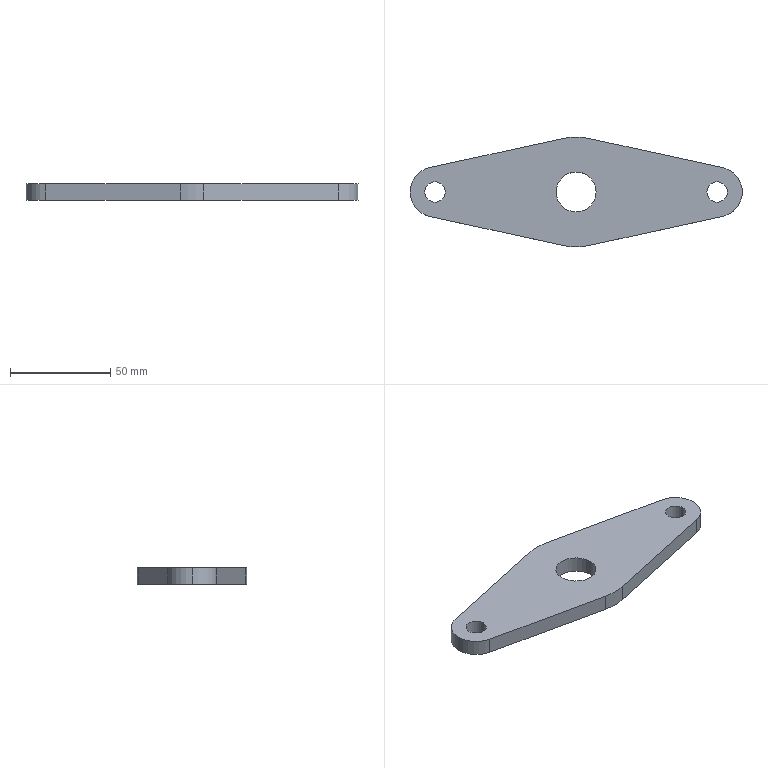Part | SolidWorks | features Extrusion 1, HoleWzd 1, ICE 1 | 1 solid | 17 faces | box 166 x 55 x 8 mm | volume 46251 mm3 | cylinder 11 | plane 6 | commonest cylinder face diameters 10.2 x4 25 x3 20 x2 55 x2
STEP:
#1=CARTESIAN_POINT('',(-10.,0.,0.));
#2=VERTEX_POINT('',#1);
#3=CARTESIAN_POINT('',(10.,0.,0.));
#4=VERTEX_POINT('',#3);
#5=CARTESIAN_POINT('',(0.,0.,0.));
#6=DIRECTION('',(0.,0.,1.));
#7=DIRECTION('',(1.,0.,0.));
#8=AXIS2_PLACEMENT_3D('',#5,#6,#7);
#9=CIRCLE('',#8,10.);
#10=EDGE_CURVE('',#2,#4,#9,.T.);
#11=ORIENTED_EDGE('',*,*,#10,.F.);
#12=CARTESIAN_POINT('',(-10.,0.,8.));
#13=VERTEX_POINT('',#12);
#14=CARTESIAN_POINT('',(-10.,0.,0.));
#15=DIRECTION('',(0.,0.,1.));
#16=VECTOR('',#15,1000.);
#17=LINE('',#14,#16);
#18=EDGE_CURVE('',#2,#13,#17,.T.);
#19=ORIENTED_EDGE('',*,*,#18,.T.);
#20=CARTESIAN_POINT('',(10.,0.,8.));
#21=VERTEX_POINT('',#20);
#22=CARTESIAN_POINT('',(0.,0.,8.));
#23=DIRECTION('',(0.,0.,1.));
#24=DIRECTION('',(1.,0.,0.));
#25=AXIS2_PLACEMENT_3D('',#22,#23,#24);
#26=CIRCLE('',#25,10.);
#27=EDGE_CURVE('',#13,#21,#26,.T.);
#28=ORIENTED_EDGE('',*,*,#27,.T.);
#29=CARTESIAN_POINT('',(10.,0.,0.));
#30=DIRECTION('',(0.,0.,1.));
#31=VECTOR('',#30,1000.);
#32=LINE('',#29,#31);
#33=EDGE_CURVE('',#4,#21,#32,.T.);
#34=ORIENTED_EDGE('',*,*,#33,.F.);
#35=EDGE_LOOP('',(#11,#19,#28,#34));
#36=FACE_OUTER_BOUND('',#35,.T.);
#37=CARTESIAN_POINT('',(0.,0.,0.));
#38=DIRECTION('',(0.,0.,1.));
#39=DIRECTION('',(1.,0.,0.));
#40=AXIS2_PLACEMENT_3D('',#37,#38,#39);
#41=CYLINDRICAL_SURFACE('',#40,10.);
#42=ADVANCED_FACE('',(#36),#41,.F.);
#43=CARTESIAN_POINT('',(-75.6,0.,0.));
#44=VERTEX_POINT('',#43);
#45=CARTESIAN_POINT('',(-65.4,0.,0.));
#46=VERTEX_POINT('',#45);
#47=CARTESIAN_POINT('',(-70.5,0.,0.));
#48=DIRECTION('',(0.,0.,1.));
#49=DIRECTION('',(1.,0.,0.));
#50=AXIS2_PLACEMENT_3D('',#47,#48,#49);
#51=CIRCLE('',#50,5.1);
#52=EDGE_CURVE('',#44,#46,#51,.T.);
#53=ORIENTED_EDGE('',*,*,#52,.F.);
#54=CARTESIAN_POINT('',(-75.6,0.,8.));
#55=VERTEX_POINT('',#54);
#56=CARTESIAN_POINT('',(-75.6,0.,8.));
#57=DIRECTION('',(0.,0.,1.));
#58=VECTOR('',#57,1000.);
#59=LINE('',#56,#58);
#60=EDGE_CURVE('',#44,#55,#59,.T.);
#61=ORIENTED_EDGE('',*,*,#60,.T.);
#62=CARTESIAN_POINT('',(-65.4,0.,8.));
#63=VERTEX_POINT('',#62);
#64=CARTESIAN_POINT('',(-70.5,0.,8.));
#65=DIRECTION('',(0.,0.,1.));
#66=DIRECTION('',(1.,0.,0.));
#67=AXIS2_PLACEMENT_3D('',#64,#65,#66);
#68=CIRCLE('',#67,5.1);
#69=EDGE_CURVE('',#55,#63,#68,.T.);
#70=ORIENTED_EDGE('',*,*,#69,.T.);
#71=CARTESIAN_POINT('',(-65.4,0.,8.));
#72=DIRECTION('',(0.,0.,1.));
#73=VECTOR('',#72,1000.);
#74=LINE('',#71,#73);
#75=EDGE_CURVE('',#46,#63,#74,.T.);
#76=ORIENTED_EDGE('',*,*,#75,.F.);
#77=EDGE_LOOP('',(#53,#61,#70,#76));
#78=FACE_OUTER_BOUND('',#77,.T.);
#79=CARTESIAN_POINT('',(-70.5,0.,8.));
#80=DIRECTION('',(0.,0.,1.));
#81=DIRECTION('',(1.,0.,0.));
#82=AXIS2_PLACEMENT_3D('',#79,#80,#81);
#83=CYLINDRICAL_SURFACE('',#82,5.1);
#84=ADVANCED_FACE('',(#78),#83,.F.);
#85=CARTESIAN_POINT('',(65.4,0.,0.));
#86=VERTEX_POINT('',#85);
#87=CARTESIAN_POINT('',(75.6,0.,0.));
#88=VERTEX_POINT('',#87);
#89=CARTESIAN_POINT('',(70.5,0.,0.));
#90=DIRECTION('',(0.,0.,1.));
#91=DIRECTION('',(1.,0.,0.));
#92=AXIS2_PLACEMENT_3D('',#89,#90,#91);
#93=CIRCLE('',#92,5.1);
#94=EDGE_CURVE('',#86,#88,#93,.T.);
#95=ORIENTED_EDGE('',*,*,#94,.F.);
#96=CARTESIAN_POINT('',(65.4,0.,8.));
#97=VERTEX_POINT('',#96);
#98=CARTESIAN_POINT('',(65.4,0.,8.));
#99=DIRECTION('',(0.,0.,1.));
#100=VECTOR('',#99,1000.);
#101=LINE('',#98,#100);
#102=EDGE_CURVE('',#86,#97,#101,.T.);
#103=ORIENTED_EDGE('',*,*,#102,.T.);
#104=CARTESIAN_POINT('',(75.6,0.,8.));
#105=VERTEX_POINT('',#104);
#106=CARTESIAN_POINT('',(70.5,0.,8.));
#107=DIRECTION('',(0.,0.,1.));
#108=DIRECTION('',(1.,0.,0.));
#109=AXIS2_PLACEMENT_3D('',#106,#107,#108);
#110=CIRCLE('',#109,5.1);
#111=EDGE_CURVE('',#97,#105,#110,.T.);
#112=ORIENTED_EDGE('',*,*,#111,.T.);
#113=CARTESIAN_POINT('',(75.6,0.,8.));
#114=DIRECTION('',(0.,0.,1.));
#115=VECTOR('',#114,1000.);
#116=LINE('',#113,#115);
#117=EDGE_CURVE('',#88,#105,#116,.T.);
#118=ORIENTED_EDGE('',*,*,#117,.F.);
#119=EDGE_LOOP('',(#95,#103,#112,#118));
#120=FACE_OUTER_BOUND('',#119,.T.);
#121=CARTESIAN_POINT('',(70.5,0.,8.));
#122=DIRECTION('',(0.,0.,1.));
#123=DIRECTION('',(1.,0.,0.));
#124=AXIS2_PLACEMENT_3D('',#121,#122,#123);
#125=CYLINDRICAL_SURFACE('',#124,5.1);
#126=ADVANCED_FACE('',(#120),#125,.F.);
#127=CARTESIAN_POINT('',(-83.,0.,8.));
#128=VERTEX_POINT('',#127);
#129=CARTESIAN_POINT('',(-73.16,-12.214,8.));
#130=VERTEX_POINT('',#129);
#131=CARTESIAN_POINT('',(-70.5,0.,8.));
#132=DIRECTION('',(0.,0.,1.));
#133=DIRECTION('',(1.,0.,0.));
#134=AXIS2_PLACEMENT_3D('',#131,#132,#133);
#135=CIRCLE('',#134,12.5);
#136=EDGE_CURVE('',#128,#130,#135,.T.);
#137=ORIENTED_EDGE('',*,*,#136,.F.);
#138=CARTESIAN_POINT('',(-83.,0.,0.));
#139=VERTEX_POINT('',#138);
#140=CARTESIAN_POINT('',(-83.,0.,8.));
#141=DIRECTION('',(0.,0.,-1.));
#142=VECTOR('',#141,1000.);
#143=LINE('',#140,#142);
#144=EDGE_CURVE('',#128,#139,#143,.T.);
#145=ORIENTED_EDGE('',*,*,#144,.T.);
#146=CARTESIAN_POINT('',(-73.16,-12.214,0.));
#147=VERTEX_POINT('',#146);
#148=CARTESIAN_POINT('',(-70.5,0.,0.));
#149=DIRECTION('',(0.,0.,1.));
#150=DIRECTION('',(1.,0.,0.));
#151=AXIS2_PLACEMENT_3D('',#148,#149,#150);
#152=CIRCLE('',#151,12.5);
#153=EDGE_CURVE('',#139,#147,#152,.T.);
#154=ORIENTED_EDGE('',*,*,#153,.T.);
#155=CARTESIAN_POINT('',(-73.16,-12.214,8.));
#156=DIRECTION('',(0.,0.,-1.));
#157=VECTOR('',#156,1000.);
#158=LINE('',#155,#157);
#159=EDGE_CURVE('',#130,#147,#158,.T.);
#160=ORIENTED_EDGE('',*,*,#159,.F.);
#161=EDGE_LOOP('',(#137,#145,#154,#160));
#162=FACE_OUTER_BOUND('',#161,.T.);
#163=CARTESIAN_POINT('',(-70.5,0.,8.));
#164=DIRECTION('',(0.,0.,-1.));
#165=DIRECTION('',(-1.,0.,0.));
#166=AXIS2_PLACEMENT_3D('',#163,#164,#165);
#167=CYLINDRICAL_SURFACE('',#166,12.5);
#168=ADVANCED_FACE('',(#162),#167,.T.);
#169=CARTESIAN_POINT('',(5.851,-26.87,0.));
#170=VERTEX_POINT('',#169);
#171=CARTESIAN_POINT('',(73.16,-12.214,0.));
#172=VERTEX_POINT('',#171);
#173=CARTESIAN_POINT('',(5.851,-26.87,0.));
#174=DIRECTION('',(0.9771,0.2128,0.));
#175=VECTOR('',#174,1000.);
#176=LINE('',#173,#175);
#177=EDGE_CURVE('',#170,#172,#176,.T.);
#178=ORIENTED_EDGE('',*,*,#177,.T.);
#179=CARTESIAN_POINT('',(73.16,-12.214,8.));
#180=VERTEX_POINT('',#179);
#181=CARTESIAN_POINT('',(73.16,-12.214,8.));
#182=DIRECTION('',(0.,0.,-1.));
#183=VECTOR('',#182,1000.);
#184=LINE('',#181,#183);
#185=EDGE_CURVE('',#180,#172,#184,.T.);
#186=ORIENTED_EDGE('',*,*,#185,.F.);
#187=CARTESIAN_POINT('',(5.851,-26.87,8.));
#188=VERTEX_POINT('',#187);
#189=CARTESIAN_POINT('',(5.851,-26.87,8.));
#190=DIRECTION('',(0.9771,0.2128,0.));
#191=VECTOR('',#190,1000.);
#192=LINE('',#189,#191);
#193=EDGE_CURVE('',#188,#180,#192,.T.);
#194=ORIENTED_EDGE('',*,*,#193,.F.);
#195=CARTESIAN_POINT('',(5.851,-26.87,8.));
#196=DIRECTION('',(0.,0.,-1.));
#197=VECTOR('',#196,1000.);
#198=LINE('',#195,#197);
#199=EDGE_CURVE('',#188,#170,#198,.T.);
#200=ORIENTED_EDGE('',*,*,#199,.T.);
#201=EDGE_LOOP('',(#178,#186,#194,#200));
#202=FACE_OUTER_BOUND('',#201,.T.);
#203=CARTESIAN_POINT('',(5.851,-26.87,8.));
#204=DIRECTION('',(-0.2128,0.9771,0.));
#205=DIRECTION('',(-0.9771,-0.2128,0.));
#206=AXIS2_PLACEMENT_3D('',#203,#204,#205);
#207=PLANE('',#206);
#208=ADVANCED_FACE('',(#202),#207,.F.);
#209=CARTESIAN_POINT('',(73.16,12.214,0.));
#210=VERTEX_POINT('',#209);
#211=CARTESIAN_POINT('',(70.5,0.,0.));
#212=DIRECTION('',(0.,0.,1.));
#213=DIRECTION('',(1.,0.,0.));
#214=AXIS2_PLACEMENT_3D('',#211,#212,#213);
#215=CIRCLE('',#214,12.5);
#216=EDGE_CURVE('',#172,#210,#215,.T.);
#217=ORIENTED_EDGE('',*,*,#216,.T.);
#218=CARTESIAN_POINT('',(73.16,12.214,8.));
#219=VERTEX_POINT('',#218);
#220=CARTESIAN_POINT('',(73.16,12.214,8.));
#221=DIRECTION('',(0.,0.,-1.));
#222=VECTOR('',#221,1000.);
#223=LINE('',#220,#222);
#224=EDGE_CURVE('',#219,#210,#223,.T.);
#225=ORIENTED_EDGE('',*,*,#224,.F.);
#226=CARTESIAN_POINT('',(70.5,0.,8.));
#227=DIRECTION('',(0.,0.,1.));
#228=DIRECTION('',(1.,0.,0.));
#229=AXIS2_PLACEMENT_3D('',#226,#227,#228);
#230=CIRCLE('',#229,12.5);
#231=EDGE_CURVE('',#180,#219,#230,.T.);
#232=ORIENTED_EDGE('',*,*,#231,.F.);
#233=ORIENTED_EDGE('',*,*,#185,.T.);
#234=EDGE_LOOP('',(#217,#225,#232,#233));
#235=FACE_OUTER_BOUND('',#234,.T.);
#236=CARTESIAN_POINT('',(70.5,0.,8.));
#237=DIRECTION('',(0.,0.,-1.));
#238=DIRECTION('',(-1.,0.,0.));
#239=AXIS2_PLACEMENT_3D('',#236,#237,#238);
#240=CYLINDRICAL_SURFACE('',#239,12.5);
#241=ADVANCED_FACE('',(#235),#240,.T.);
#242=CARTESIAN_POINT('',(5.851,26.87,0.));
#243=VERTEX_POINT('',#242);
#244=CARTESIAN_POINT('',(5.851,26.87,0.));
#245=DIRECTION('',(0.9771,-0.2128,0.));
#246=VECTOR('',#245,1000.);
#247=LINE('',#244,#246);
#248=EDGE_CURVE('',#243,#210,#247,.T.);
#249=ORIENTED_EDGE('',*,*,#248,.F.);
#250=CARTESIAN_POINT('',(5.851,26.87,8.));
#251=VERTEX_POINT('',#250);
#252=CARTESIAN_POINT('',(5.851,26.87,8.));
#253=DIRECTION('',(0.,0.,-1.));
#254=VECTOR('',#253,1000.);
#255=LINE('',#252,#254);
#256=EDGE_CURVE('',#251,#243,#255,.T.);
#257=ORIENTED_EDGE('',*,*,#256,.F.);
#258=CARTESIAN_POINT('',(5.851,26.87,8.));
#259=DIRECTION('',(0.9771,-0.2128,0.));
#260=VECTOR('',#259,1000.);
#261=LINE('',#258,#260);
#262=EDGE_CURVE('',#251,#219,#261,.T.);
#263=ORIENTED_EDGE('',*,*,#262,.T.);
#264=ORIENTED_EDGE('',*,*,#224,.T.);
#265=EDGE_LOOP('',(#249,#257,#263,#264));
#266=FACE_OUTER_BOUND('',#265,.T.);
#267=CARTESIAN_POINT('',(5.851,26.87,8.));
#268=DIRECTION('',(0.2128,0.9771,0.));
#269=DIRECTION('',(-0.9771,0.2128,0.));
#270=AXIS2_PLACEMENT_3D('',#267,#268,#269);
#271=PLANE('',#270);
#272=ADVANCED_FACE('',(#266),#271,.T.);
#273=CARTESIAN_POINT('',(-5.851,26.87,0.));
#274=VERTEX_POINT('',#273);
#275=CARTESIAN_POINT('',(0.,0.,0.));
#276=DIRECTION('',(0.,0.,1.));
#277=DIRECTION('',(1.,0.,0.));
#278=AXIS2_PLACEMENT_3D('',#275,#276,#277);
#279=CIRCLE('',#278,27.5);
#280=EDGE_CURVE('',#243,#274,#279,.T.);
#281=ORIENTED_EDGE('',*,*,#280,.T.);
#282=CARTESIAN_POINT('',(-5.851,26.87,8.));
#283=VERTEX_POINT('',#282);
#284=CARTESIAN_POINT('',(-5.851,26.87,8.));
#285=DIRECTION('',(0.,0.,-1.));
#286=VECTOR('',#285,1000.);
#287=LINE('',#284,#286);
#288=EDGE_CURVE('',#283,#274,#287,.T.);
#289=ORIENTED_EDGE('',*,*,#288,.F.);
#290=CARTESIAN_POINT('',(0.,0.,8.));
#291=DIRECTION('',(0.,0.,1.));
#292=DIRECTION('',(1.,0.,0.));
#293=AXIS2_PLACEMENT_3D('',#290,#291,#292);
#294=CIRCLE('',#293,27.5);
#295=EDGE_CURVE('',#251,#283,#294,.T.);
#296=ORIENTED_EDGE('',*,*,#295,.F.);
#297=ORIENTED_EDGE('',*,*,#256,.T.);
#298=EDGE_LOOP('',(#281,#289,#296,#297));
#299=FACE_OUTER_BOUND('',#298,.T.);
#300=CARTESIAN_POINT('',(0.,0.,8.));
#301=DIRECTION('',(0.,0.,-1.));
#302=DIRECTION('',(-1.,0.,0.));
#303=AXIS2_PLACEMENT_3D('',#300,#301,#302);
#304=CYLINDRICAL_SURFACE('',#303,27.5);
#305=ADVANCED_FACE('',(#299),#304,.T.);
#306=CARTESIAN_POINT('',(-73.16,12.214,0.));
#307=VERTEX_POINT('',#306);
#308=CARTESIAN_POINT('',(-73.16,12.214,0.));
#309=DIRECTION('',(0.9771,0.2128,0.));
#310=VECTOR('',#309,1000.);
#311=LINE('',#308,#310);
#312=EDGE_CURVE('',#307,#274,#311,.T.);
#313=ORIENTED_EDGE('',*,*,#312,.F.);
#314=CARTESIAN_POINT('',(-73.16,12.214,8.));
#315=VERTEX_POINT('',#314);
#316=CARTESIAN_POINT('',(-73.16,12.214,8.));
#317=DIRECTION('',(0.,0.,-1.));
#318=VECTOR('',#317,1000.);
#319=LINE('',#316,#318);
#320=EDGE_CURVE('',#315,#307,#319,.T.);
#321=ORIENTED_EDGE('',*,*,#320,.F.);
#322=CARTESIAN_POINT('',(-73.16,12.214,8.));
#323=DIRECTION('',(0.9771,0.2128,0.));
#324=VECTOR('',#323,1000.);
#325=LINE('',#322,#324);
#326=EDGE_CURVE('',#315,#283,#325,.T.);
#327=ORIENTED_EDGE('',*,*,#326,.T.);
#328=ORIENTED_EDGE('',*,*,#288,.T.);
#329=EDGE_LOOP('',(#313,#321,#327,#328));
#330=FACE_OUTER_BOUND('',#329,.T.);
#331=CARTESIAN_POINT('',(-73.16,12.214,8.));
#332=DIRECTION('',(-0.2128,0.9771,0.));
#333=DIRECTION('',(-0.9771,-0.2128,0.));
#334=AXIS2_PLACEMENT_3D('',#331,#332,#333);
#335=PLANE('',#334);
#336=ADVANCED_FACE('',(#330),#335,.T.);
#337=ORIENTED_EDGE('',*,*,#144,.F.);
#338=CARTESIAN_POINT('',(-70.5,0.,8.));
#339=DIRECTION('',(0.,0.,1.));
#340=DIRECTION('',(1.,0.,0.));
#341=AXIS2_PLACEMENT_3D('',#338,#339,#340);
#342=CIRCLE('',#341,12.5);
#343=EDGE_CURVE('',#315,#128,#342,.T.);
#344=ORIENTED_EDGE('',*,*,#343,.F.);
#345=ORIENTED_EDGE('',*,*,#320,.T.);
#346=CARTESIAN_POINT('',(-70.5,0.,0.));
#347=DIRECTION('',(0.,0.,1.));
#348=DIRECTION('',(1.,0.,0.));
#349=AXIS2_PLACEMENT_3D('',#346,#347,#348);
#350=CIRCLE('',#349,12.5);
#351=EDGE_CURVE('',#307,#139,#350,.T.);
#352=ORIENTED_EDGE('',*,*,#351,.T.);
#353=EDGE_LOOP('',(#337,#344,#345,#352));
#354=FACE_OUTER_BOUND('',#353,.T.);
#355=CARTESIAN_POINT('',(-70.5,0.,8.));
#356=DIRECTION('',(0.,0.,-1.));
#357=DIRECTION('',(-1.,0.,0.));
#358=AXIS2_PLACEMENT_3D('',#355,#356,#357);
#359=CYLINDRICAL_SURFACE('',#358,12.5);
#360=ADVANCED_FACE('',(#354),#359,.T.);
#361=CARTESIAN_POINT('',(-5.851,-26.87,0.));
#362=VERTEX_POINT('',#361);
#363=CARTESIAN_POINT('',(-73.16,-12.214,0.));
#364=DIRECTION('',(0.9771,-0.2128,0.));
#365=VECTOR('',#364,1000.);
#366=LINE('',#363,#365);
#367=EDGE_CURVE('',#147,#362,#366,.T.);
#368=ORIENTED_EDGE('',*,*,#367,.T.);
#369=CARTESIAN_POINT('',(-5.851,-26.87,8.));
#370=VERTEX_POINT('',#369);
#371=CARTESIAN_POINT('',(-5.851,-26.87,8.));
#372=DIRECTION('',(0.,0.,-1.));
#373=VECTOR('',#372,1000.);
#374=LINE('',#371,#373);
#375=EDGE_CURVE('',#370,#362,#374,.T.);
#376=ORIENTED_EDGE('',*,*,#375,.F.);
#377=CARTESIAN_POINT('',(-73.16,-12.214,8.));
#378=DIRECTION('',(0.9771,-0.2128,0.));
#379=VECTOR('',#378,1000.);
#380=LINE('',#377,#379);
#381=EDGE_CURVE('',#130,#370,#380,.T.);
#382=ORIENTED_EDGE('',*,*,#381,.F.);
#383=ORIENTED_EDGE('',*,*,#159,.T.);
#384=EDGE_LOOP('',(#368,#376,#382,#383));
#385=FACE_OUTER_BOUND('',#384,.T.);
#386=CARTESIAN_POINT('',(-73.16,-12.214,8.));
#387=DIRECTION('',(0.2128,0.9771,0.));
#388=DIRECTION('',(-0.9771,0.2128,0.));
#389=AXIS2_PLACEMENT_3D('',#386,#387,#388);
#390=PLANE('',#389);
#391=ADVANCED_FACE('',(#385),#390,.F.);
#392=CARTESIAN_POINT('',(0.,0.,0.));
#393=DIRECTION('',(0.,0.,1.));
#394=DIRECTION('',(1.,0.,0.));
#395=AXIS2_PLACEMENT_3D('',#392,#393,#394);
#396=CIRCLE('',#395,27.5);
#397=EDGE_CURVE('',#362,#170,#396,.T.);
#398=ORIENTED_EDGE('',*,*,#397,.T.);
#399=ORIENTED_EDGE('',*,*,#199,.F.);
#400=CARTESIAN_POINT('',(0.,0.,8.));
#401=DIRECTION('',(0.,0.,1.));
#402=DIRECTION('',(1.,0.,0.));
#403=AXIS2_PLACEMENT_3D('',#400,#401,#402);
#404=CIRCLE('',#403,27.5);
#405=EDGE_CURVE('',#370,#188,#404,.T.);
#406=ORIENTED_EDGE('',*,*,#405,.F.);
#407=ORIENTED_EDGE('',*,*,#375,.T.);
#408=EDGE_LOOP('',(#398,#399,#406,#407));
#409=FACE_OUTER_BOUND('',#408,.T.);
#410=CARTESIAN_POINT('',(0.,0.,8.));
#411=DIRECTION('',(0.,0.,-1.));
#412=DIRECTION('',(-1.,0.,0.));
#413=AXIS2_PLACEMENT_3D('',#410,#411,#412);
#414=CYLINDRICAL_SURFACE('',#413,27.5);
#415=ADVANCED_FACE('',(#409),#414,.T.);
#416=CARTESIAN_POINT('',(0.,0.,8.));
#417=DIRECTION('',(0.,0.,1.));
#418=DIRECTION('',(1.,0.,0.));
#419=AXIS2_PLACEMENT_3D('',#416,#417,#418);
#420=CIRCLE('',#419,10.);
#421=EDGE_CURVE('',#21,#13,#420,.T.);
#422=ORIENTED_EDGE('',*,*,#421,.F.);
#423=ORIENTED_EDGE('',*,*,#27,.F.);
#424=EDGE_LOOP('',(#422,#423));
#425=FACE_BOUND('',#424,.T.);
#426=CARTESIAN_POINT('',(-70.5,0.,8.));
#427=DIRECTION('',(0.,0.,1.));
#428=DIRECTION('',(1.,0.,0.));
#429=AXIS2_PLACEMENT_3D('',#426,#427,#428);
#430=CIRCLE('',#429,5.1);
#431=EDGE_CURVE('',#63,#55,#430,.T.);
#432=ORIENTED_EDGE('',*,*,#431,.F.);
#433=ORIENTED_EDGE('',*,*,#69,.F.);
#434=EDGE_LOOP('',(#432,#433));
#435=FACE_BOUND('',#434,.T.);
#436=CARTESIAN_POINT('',(70.5,0.,8.));
#437=DIRECTION('',(0.,0.,1.));
#438=DIRECTION('',(1.,0.,0.));
#439=AXIS2_PLACEMENT_3D('',#436,#437,#438);
#440=CIRCLE('',#439,5.1);
#441=EDGE_CURVE('',#105,#97,#440,.T.);
#442=ORIENTED_EDGE('',*,*,#441,.F.);
#443=ORIENTED_EDGE('',*,*,#111,.F.);
#444=EDGE_LOOP('',(#442,#443));
#445=FACE_BOUND('',#444,.T.);
#446=ORIENTED_EDGE('',*,*,#193,.T.);
#447=ORIENTED_EDGE('',*,*,#231,.T.);
#448=ORIENTED_EDGE('',*,*,#262,.F.);
#449=ORIENTED_EDGE('',*,*,#295,.T.);
#450=ORIENTED_EDGE('',*,*,#326,.F.);
#451=ORIENTED_EDGE('',*,*,#343,.T.);
#452=ORIENTED_EDGE('',*,*,#136,.T.);
#453=ORIENTED_EDGE('',*,*,#381,.T.);
#454=ORIENTED_EDGE('',*,*,#405,.T.);
#455=EDGE_LOOP('',(#446,#447,#448,#449,#450,#451,#452,#453,#454));
#456=FACE_OUTER_BOUND('',#455,.T.);
#457=CARTESIAN_POINT('',(70.5,0.,8.));
#458=DIRECTION('',(0.,0.,1.));
#459=DIRECTION('',(1.,0.,0.));
#460=AXIS2_PLACEMENT_3D('',#457,#458,#459);
#461=PLANE('',#460);
#462=ADVANCED_FACE('',(#425,#435,#445,#456),#461,.T.);
#463=CARTESIAN_POINT('',(0.,0.,0.));
#464=DIRECTION('',(0.,0.,1.));
#465=DIRECTION('',(1.,0.,0.));
#466=AXIS2_PLACEMENT_3D('',#463,#464,#465);
#467=CIRCLE('',#466,10.);
#468=EDGE_CURVE('',#4,#2,#467,.T.);
#469=ORIENTED_EDGE('',*,*,#468,.T.);
#470=ORIENTED_EDGE('',*,*,#10,.T.);
#471=EDGE_LOOP('',(#469,#470));
#472=FACE_BOUND('',#471,.T.);
#473=CARTESIAN_POINT('',(-70.5,0.,0.));
#474=DIRECTION('',(0.,0.,1.));
#475=DIRECTION('',(1.,0.,0.));
#476=AXIS2_PLACEMENT_3D('',#473,#474,#475);
#477=CIRCLE('',#476,5.1);
#478=EDGE_CURVE('',#46,#44,#477,.T.);
#479=ORIENTED_EDGE('',*,*,#478,.T.);
#480=ORIENTED_EDGE('',*,*,#52,.T.);
#481=EDGE_LOOP('',(#479,#480));
#482=FACE_BOUND('',#481,.T.);
#483=CARTESIAN_POINT('',(70.5,0.,0.));
#484=DIRECTION('',(0.,0.,1.));
#485=DIRECTION('',(1.,0.,0.));
#486=AXIS2_PLACEMENT_3D('',#483,#484,#485);
#487=CIRCLE('',#486,5.1);
#488=EDGE_CURVE('',#88,#86,#487,.T.);
#489=ORIENTED_EDGE('',*,*,#488,.T.);
#490=ORIENTED_EDGE('',*,*,#94,.T.);
#491=EDGE_LOOP('',(#489,#490));
#492=FACE_BOUND('',#491,.T.);
#493=ORIENTED_EDGE('',*,*,#177,.F.);
#494=ORIENTED_EDGE('',*,*,#397,.F.);
#495=ORIENTED_EDGE('',*,*,#367,.F.);
#496=ORIENTED_EDGE('',*,*,#153,.F.);
#497=ORIENTED_EDGE('',*,*,#351,.F.);
#498=ORIENTED_EDGE('',*,*,#312,.T.);
#499=ORIENTED_EDGE('',*,*,#280,.F.);
#500=ORIENTED_EDGE('',*,*,#248,.T.);
#501=ORIENTED_EDGE('',*,*,#216,.F.);
#502=EDGE_LOOP('',(#493,#494,#495,#496,#497,#498,#499,#500,#501));
#503=FACE_OUTER_BOUND('',#502,.T.);
#504=CARTESIAN_POINT('',(70.5,0.,0.));
#505=DIRECTION('',(0.,0.,1.));
#506=DIRECTION('',(1.,0.,0.));
#507=AXIS2_PLACEMENT_3D('',#504,#505,#506);
#508=PLANE('',#507);
#509=ADVANCED_FACE('',(#472,#482,#492,#503),#508,.F.);
#510=ORIENTED_EDGE('',*,*,#102,.F.);
#511=ORIENTED_EDGE('',*,*,#488,.F.);
#512=ORIENTED_EDGE('',*,*,#117,.T.);
#513=ORIENTED_EDGE('',*,*,#441,.T.);
#514=EDGE_LOOP('',(#510,#511,#512,#513));
#515=FACE_OUTER_BOUND('',#514,.T.);
#516=CARTESIAN_POINT('',(70.5,0.,8.));
#517=DIRECTION('',(0.,0.,1.));
#518=DIRECTION('',(1.,0.,0.));
#519=AXIS2_PLACEMENT_3D('',#516,#517,#518);
#520=CYLINDRICAL_SURFACE('',#519,5.1);
#521=ADVANCED_FACE('',(#515),#520,.F.);
#522=ORIENTED_EDGE('',*,*,#60,.F.);
#523=ORIENTED_EDGE('',*,*,#478,.F.);
#524=ORIENTED_EDGE('',*,*,#75,.T.);
#525=ORIENTED_EDGE('',*,*,#431,.T.);
#526=EDGE_LOOP('',(#522,#523,#524,#525));
#527=FACE_OUTER_BOUND('',#526,.T.);
#528=CARTESIAN_POINT('',(-70.5,0.,8.));
#529=DIRECTION('',(0.,0.,1.));
#530=DIRECTION('',(1.,0.,0.));
#531=AXIS2_PLACEMENT_3D('',#528,#529,#530);
#532=CYLINDRICAL_SURFACE('',#531,5.1);
#533=ADVANCED_FACE('',(#527),#532,.F.);
#534=ORIENTED_EDGE('',*,*,#18,.F.);
#535=ORIENTED_EDGE('',*,*,#468,.F.);
#536=ORIENTED_EDGE('',*,*,#33,.T.);
#537=ORIENTED_EDGE('',*,*,#421,.T.);
#538=EDGE_LOOP('',(#534,#535,#536,#537));
#539=FACE_OUTER_BOUND('',#538,.T.);
#540=CARTESIAN_POINT('',(0.,0.,0.));
#541=DIRECTION('',(0.,0.,1.));
#542=DIRECTION('',(1.,0.,0.));
#543=AXIS2_PLACEMENT_3D('',#540,#541,#542);
#544=CYLINDRICAL_SURFACE('',#543,10.);
#545=ADVANCED_FACE('',(#539),#544,.F.);
#546=CLOSED_SHELL('',(#42,#84,#126,#168,#208,#241,#272,#305,#336,#360,#391,#415,#462,#509,#521,#533,#545));
#547=MANIFOLD_SOLID_BREP('',#546);
#548=CARTESIAN_POINT('',(0.,0.,0.));
#549=DIRECTION('',(0.,0.,1.));
#550=DIRECTION('',(1.,0.,0.));
#551=AXIS2_PLACEMENT_3D('',#548,#549,#550);
#552=(LENGTH_UNIT()NAMED_UNIT(*)SI_UNIT(.MILLI.,.METRE.));
#553=UNCERTAINTY_MEASURE_WITH_UNIT(LENGTH_MEASURE(0.00001),#552,'','');
#554=(NAMED_UNIT(*)PLANE_ANGLE_UNIT()SI_UNIT($,.RADIAN.));
#555=(NAMED_UNIT(*)SI_UNIT($,.STERADIAN.)SOLID_ANGLE_UNIT());
#556=(GEOMETRIC_REPRESENTATION_CONTEXT(3)GLOBAL_UNCERTAINTY_ASSIGNED_CONTEXT((#553))GLOBAL_UNIT_ASSIGNED_CONTEXT((#552,#554,#555))REPRESENTATION_CONTEXT('',''));
#557=ADVANCED_BREP_SHAPE_REPRESENTATION('',(#547,#551),#556);